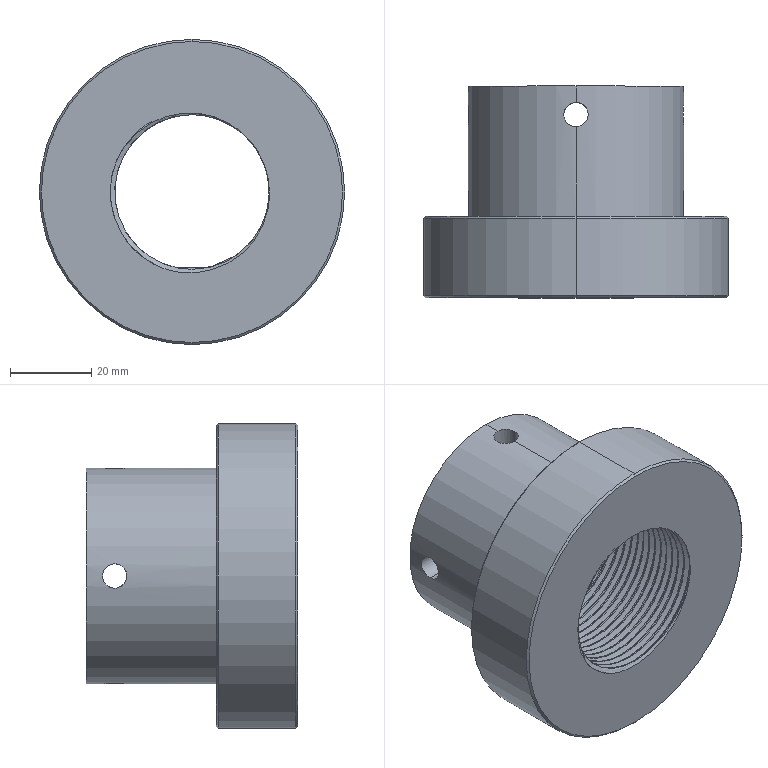Part | SolidWorks | features BaseBody 1 | 1 solid | 115 faces | box 75 x 52 x 75 mm | volume 95331 mm3 | cylinder 71 | spline 36 | cone 4 | plane 4 | commonest cylinder face diameters 38 x59 6 x8 53 x2 75 x2